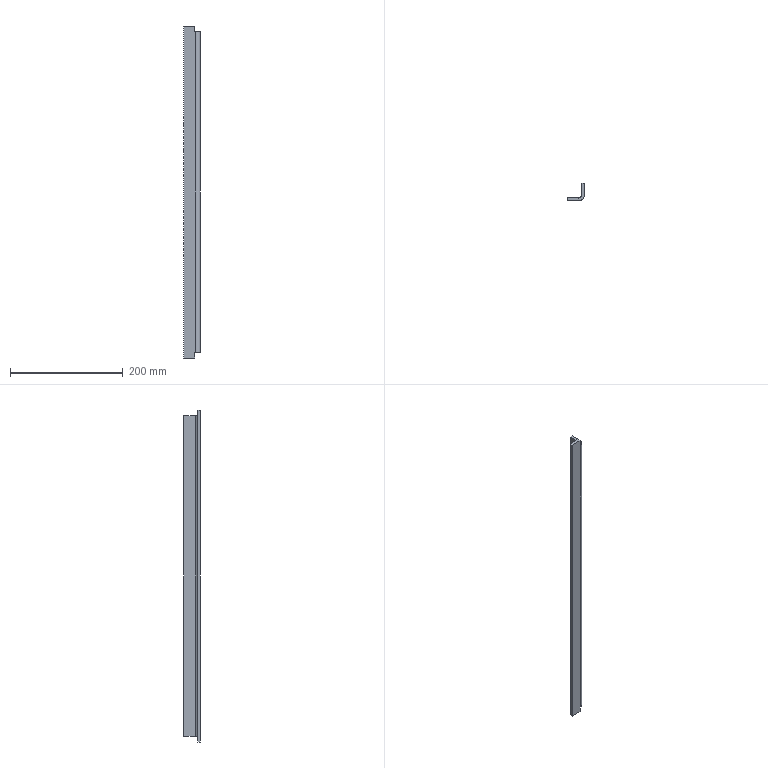Part | STEP file | PN_0019_bent angle steel | 1 solid | 14 faces | box 30 x 30 x 590 mm | volume 150799 mm3 | plane 12 | cylinder 2 | commonest cylinder face diameters 8 x1 18 x1
STEP:
#1=CARTESIAN_POINT('',(0.,0.,0.));
#2=DIRECTION('',(0.,0.,1.));
#3=DIRECTION('',(1.,0.,0.));
#4=AXIS2_PLACEMENT_3D('',#1,#2,#3);
#5=CARTESIAN_POINT('',(189.,-130.,10.));
#6=VERTEX_POINT('',#5);
#7=CARTESIAN_POINT('',(188.,-130.,10.));
#8=VERTEX_POINT('',#7);
#9=CARTESIAN_POINT('',(188.,-130.,10.));
#10=DIRECTION('',(-1.,0.,0.));
#11=VECTOR('',#10,1.);
#12=LINE('',#9,#11);
#13=CARTESIAN_POINT('',(198.,-130.,295.));
#14=DIRECTION('',(0.,-1.,0.));
#15=DIRECTION('',(0.,0.,-1.));
#16=AXIS2_PLACEMENT_3D('',#13,#14,#15);
#17=PLANE('',#16);
#18=CARTESIAN_POINT('',(285.,-10.));
#19=DIRECTION('',(0.,-1.));
#20=VECTOR('',#19,1.);
#21=LINE('',#18,#20);
#22=(GEOMETRIC_REPRESENTATION_CONTEXT(2)PARAMETRIC_REPRESENTATION_CONTEXT()REPRESENTATION_CONTEXT('',''));
#23=DEFINITIONAL_REPRESENTATION('',(#21),#22);
#24=PCURVE('',#17,#23);
#25=CARTESIAN_POINT('',(188.,-105.,10.));
#26=DIRECTION('',(0.,0.,1.));
#27=DIRECTION('',(0.,-1.,0.));
#28=AXIS2_PLACEMENT_3D('',#25,#26,#27);
#29=PLANE('',#28);
#30=CARTESIAN_POINT('',(25.,0.));
#31=DIRECTION('',(0.,-1.));
#32=VECTOR('',#31,1.);
#33=LINE('',#30,#32);
#34=(GEOMETRIC_REPRESENTATION_CONTEXT(2)PARAMETRIC_REPRESENTATION_CONTEXT()REPRESENTATION_CONTEXT('',''));
#35=DEFINITIONAL_REPRESENTATION('',(#33),#34);
#36=PCURVE('',#29,#35);
#37=SURFACE_CURVE('',#12,(#24,#36),.PCURVE_S1.);
#38=EDGE_CURVE('',#6,#8,#37,.T.);
#39=ORIENTED_EDGE('',*,*,#38,.T.);
#40=CARTESIAN_POINT('',(188.,-130.,0.));
#41=VERTEX_POINT('',#40);
#42=CARTESIAN_POINT('',(188.,-130.,295.));
#43=DIRECTION('',(0.,0.,1.));
#44=VECTOR('',#43,1.);
#45=LINE('',#42,#44);
#46=CARTESIAN_POINT('',(0.,-10.));
#47=DIRECTION('',(-1.,0.));
#48=VECTOR('',#47,1.);
#49=LINE('',#46,#48);
#50=(GEOMETRIC_REPRESENTATION_CONTEXT(2)PARAMETRIC_REPRESENTATION_CONTEXT()REPRESENTATION_CONTEXT('',''));
#51=DEFINITIONAL_REPRESENTATION('',(#49),#50);
#52=PCURVE('',#17,#51);
#53=CARTESIAN_POINT('',(188.,0.,0.));
#54=DIRECTION('',(-1.,0.,0.));
#55=DIRECTION('',(0.,0.,1.));
#56=AXIS2_PLACEMENT_3D('',#53,#54,#55);
#57=PLANE('',#56);
#58=CARTESIAN_POINT('',(295.,-130.));
#59=DIRECTION('',(1.,0.));
#60=VECTOR('',#59,1.);
#61=LINE('',#58,#60);
#62=(GEOMETRIC_REPRESENTATION_CONTEXT(2)PARAMETRIC_REPRESENTATION_CONTEXT()REPRESENTATION_CONTEXT('',''));
#63=DEFINITIONAL_REPRESENTATION('',(#61),#62);
#64=PCURVE('',#57,#63);
#65=SURFACE_CURVE('',#45,(#52,#64),.PCURVE_S1.);
#66=EDGE_CURVE('',#41,#8,#65,.T.);
#67=ORIENTED_EDGE('',*,*,#66,.F.);
#68=CARTESIAN_POINT('',(168.,-130.,0.));
#69=VERTEX_POINT('',#68);
#70=CARTESIAN_POINT('',(198.,-130.,0.));
#71=DIRECTION('',(1.,0.,0.));
#72=VECTOR('',#71,1.);
#73=LINE('',#70,#72);
#74=CARTESIAN_POINT('',(295.,0.));
#75=DIRECTION('',(0.,1.));
#76=VECTOR('',#75,1.);
#77=LINE('',#74,#76);
#78=(GEOMETRIC_REPRESENTATION_CONTEXT(2)PARAMETRIC_REPRESENTATION_CONTEXT()REPRESENTATION_CONTEXT('',''));
#79=DEFINITIONAL_REPRESENTATION('',(#77),#78);
#80=PCURVE('',#17,#79);
#81=CARTESIAN_POINT('',(189.,-126.,0.));
#82=DIRECTION('',(0.,0.,1.));
#83=DIRECTION('',(0.,-1.,0.));
#84=AXIS2_PLACEMENT_3D('',#81,#82,#83);
#85=PLANE('',#84);
#86=CARTESIAN_POINT('',(4.,9.));
#87=DIRECTION('',(0.,1.));
#88=VECTOR('',#87,1.);
#89=LINE('',#86,#88);
#90=(GEOMETRIC_REPRESENTATION_CONTEXT(2)PARAMETRIC_REPRESENTATION_CONTEXT()REPRESENTATION_CONTEXT('',''));
#91=DEFINITIONAL_REPRESENTATION('',(#89),#90);
#92=PCURVE('',#85,#91);
#93=SURFACE_CURVE('',#73,(#80,#92),.PCURVE_S1.);
#94=EDGE_CURVE('',#69,#41,#93,.T.);
#95=ORIENTED_EDGE('',*,*,#94,.F.);
#96=CARTESIAN_POINT('',(168.,-130.,590.));
#97=VERTEX_POINT('',#96);
#98=CARTESIAN_POINT('',(168.,-130.,295.));
#99=DIRECTION('',(0.,0.,-1.));
#100=VECTOR('',#99,1.);
#101=LINE('',#98,#100);
#102=CARTESIAN_POINT('',(0.,-30.));
#103=DIRECTION('',(1.,0.));
#104=VECTOR('',#103,1.);
#105=LINE('',#102,#104);
#106=(GEOMETRIC_REPRESENTATION_CONTEXT(2)PARAMETRIC_REPRESENTATION_CONTEXT()REPRESENTATION_CONTEXT('',''));
#107=DEFINITIONAL_REPRESENTATION('',(#105),#106);
#108=PCURVE('',#17,#107);
#109=CARTESIAN_POINT('',(168.,-135.,295.));
#110=DIRECTION('',(-1.,0.,0.));
#111=DIRECTION('',(0.,0.,1.));
#112=AXIS2_PLACEMENT_3D('',#109,#110,#111);
#113=PLANE('',#112);
#114=CARTESIAN_POINT('',(0.,5.));
#115=DIRECTION('',(-1.,0.));
#116=VECTOR('',#115,1.);
#117=LINE('',#114,#116);
#118=(GEOMETRIC_REPRESENTATION_CONTEXT(2)PARAMETRIC_REPRESENTATION_CONTEXT()REPRESENTATION_CONTEXT('',''));
#119=DEFINITIONAL_REPRESENTATION('',(#117),#118);
#120=PCURVE('',#113,#119);
#121=SURFACE_CURVE('',#101,(#108,#120),.PCURVE_S1.);
#122=EDGE_CURVE('',#97,#69,#121,.T.);
#123=ORIENTED_EDGE('',*,*,#122,.F.);
#124=CARTESIAN_POINT('',(188.,-130.,590.));
#125=VERTEX_POINT('',#124);
#126=CARTESIAN_POINT('',(198.,-130.,590.));
#127=DIRECTION('',(-1.,0.,0.));
#128=VECTOR('',#127,1.);
#129=LINE('',#126,#128);
#130=CARTESIAN_POINT('',(-295.,0.));
#131=DIRECTION('',(0.,-1.));
#132=VECTOR('',#131,1.);
#133=LINE('',#130,#132);
#134=(GEOMETRIC_REPRESENTATION_CONTEXT(2)PARAMETRIC_REPRESENTATION_CONTEXT()REPRESENTATION_CONTEXT('',''));
#135=DEFINITIONAL_REPRESENTATION('',(#133),#134);
#136=PCURVE('',#17,#135);
#137=CARTESIAN_POINT('',(189.,-126.,590.));
#138=DIRECTION('',(0.,0.,-1.));
#139=DIRECTION('',(0.,1.,0.));
#140=AXIS2_PLACEMENT_3D('',#137,#138,#139);
#141=PLANE('',#140);
#142=CARTESIAN_POINT('',(-4.,9.));
#143=DIRECTION('',(0.,-1.));
#144=VECTOR('',#143,1.);
#145=LINE('',#142,#144);
#146=(GEOMETRIC_REPRESENTATION_CONTEXT(2)PARAMETRIC_REPRESENTATION_CONTEXT()REPRESENTATION_CONTEXT('',''));
#147=DEFINITIONAL_REPRESENTATION('',(#145),#146);
#148=PCURVE('',#141,#147);
#149=SURFACE_CURVE('',#129,(#136,#148),.PCURVE_S1.);
#150=EDGE_CURVE('',#125,#97,#149,.T.);
#151=ORIENTED_EDGE('',*,*,#150,.F.);
#152=CARTESIAN_POINT('',(188.,-130.,580.));
#153=VERTEX_POINT('',#152);
#154=CARTESIAN_POINT('',(188.,-130.,295.));
#155=DIRECTION('',(0.,0.,1.));
#156=VECTOR('',#155,1.);
#157=LINE('',#154,#156);
#158=CARTESIAN_POINT('',(0.,-10.));
#159=DIRECTION('',(-1.,0.));
#160=VECTOR('',#159,1.);
#161=LINE('',#158,#160);
#162=(GEOMETRIC_REPRESENTATION_CONTEXT(2)PARAMETRIC_REPRESENTATION_CONTEXT()REPRESENTATION_CONTEXT('',''));
#163=DEFINITIONAL_REPRESENTATION('',(#161),#162);
#164=PCURVE('',#17,#163);
#165=CARTESIAN_POINT('',(188.,0.,590.));
#166=DIRECTION('',(-1.,0.,0.));
#167=DIRECTION('',(0.,0.,1.));
#168=AXIS2_PLACEMENT_3D('',#165,#166,#167);
#169=PLANE('',#168);
#170=CARTESIAN_POINT('',(-295.,-130.));
#171=DIRECTION('',(1.,0.));
#172=VECTOR('',#171,1.);
#173=LINE('',#170,#172);
#174=(GEOMETRIC_REPRESENTATION_CONTEXT(2)PARAMETRIC_REPRESENTATION_CONTEXT()REPRESENTATION_CONTEXT('',''));
#175=DEFINITIONAL_REPRESENTATION('',(#173),#174);
#176=PCURVE('',#169,#175);
#177=SURFACE_CURVE('',#157,(#164,#176),.PCURVE_S1.);
#178=EDGE_CURVE('',#153,#125,#177,.T.);
#179=ORIENTED_EDGE('',*,*,#178,.F.);
#180=CARTESIAN_POINT('',(189.,-130.,580.));
#181=VERTEX_POINT('',#180);
#182=CARTESIAN_POINT('',(188.,-130.,580.));
#183=DIRECTION('',(1.,0.,0.));
#184=VECTOR('',#183,1.);
#185=LINE('',#182,#184);
#186=CARTESIAN_POINT('',(-285.,-10.));
#187=DIRECTION('',(0.,1.));
#188=VECTOR('',#187,1.);
#189=LINE('',#186,#188);
#190=(GEOMETRIC_REPRESENTATION_CONTEXT(2)PARAMETRIC_REPRESENTATION_CONTEXT()REPRESENTATION_CONTEXT('',''));
#191=DEFINITIONAL_REPRESENTATION('',(#189),#190);
#192=PCURVE('',#17,#191);
#193=CARTESIAN_POINT('',(188.,-105.,580.));
#194=DIRECTION('',(0.,0.,-1.));
#195=DIRECTION('',(0.,1.,0.));
#196=AXIS2_PLACEMENT_3D('',#193,#194,#195);
#197=PLANE('',#196);
#198=CARTESIAN_POINT('',(-25.,0.));
#199=DIRECTION('',(0.,1.));
#200=VECTOR('',#199,1.);
#201=LINE('',#198,#200);
#202=(GEOMETRIC_REPRESENTATION_CONTEXT(2)PARAMETRIC_REPRESENTATION_CONTEXT()REPRESENTATION_CONTEXT('',''));
#203=DEFINITIONAL_REPRESENTATION('',(#201),#202);
#204=PCURVE('',#197,#203);
#205=SURFACE_CURVE('',#185,(#192,#204),.PCURVE_S1.);
#206=EDGE_CURVE('',#153,#181,#205,.T.);
#207=ORIENTED_EDGE('',*,*,#206,.T.);
#208=CARTESIAN_POINT('',(189.,-130.,295.));
#209=DIRECTION('',(0.,0.,1.));
#210=VECTOR('',#209,1.);
#211=LINE('',#208,#210);
#212=CARTESIAN_POINT('',(0.,-9.));
#213=DIRECTION('',(-1.,0.));
#214=VECTOR('',#213,1.);
#215=LINE('',#212,#214);
#216=(GEOMETRIC_REPRESENTATION_CONTEXT(2)PARAMETRIC_REPRESENTATION_CONTEXT()REPRESENTATION_CONTEXT('',''));
#217=DEFINITIONAL_REPRESENTATION('',(#215),#216);
#218=PCURVE('',#17,#217);
#219=CARTESIAN_POINT('',(189.,-126.,295.));
#220=DIRECTION('',(0.,0.,-1.));
#221=DIRECTION('',(0.,1.,0.));
#222=AXIS2_PLACEMENT_3D('',#219,#220,#221);
#223=CYLINDRICAL_SURFACE('',#222,4.);
#224=CARTESIAN_POINT('',(3.142,0.));
#225=DIRECTION('',(0.,-1.));
#226=VECTOR('',#225,1.);
#227=LINE('',#224,#226);
#228=(GEOMETRIC_REPRESENTATION_CONTEXT(2)PARAMETRIC_REPRESENTATION_CONTEXT()REPRESENTATION_CONTEXT('',''));
#229=DEFINITIONAL_REPRESENTATION('',(#227),#228);
#230=PCURVE('',#223,#229);
#231=SURFACE_CURVE('',#211,(#218,#230),.PCURVE_S1.);
#232=EDGE_CURVE('',#6,#181,#231,.T.);
#233=ORIENTED_EDGE('',*,*,#232,.F.);
#234=EDGE_LOOP('',(#39,#67,#95,#123,#151,#179,#207,#233));
#235=FACE_BOUND('',#234,.T.);
#236=ADVANCED_FACE('',(#235),#17,.F.);
#237=CARTESIAN_POINT('',(193.,-126.,10.));
#238=VERTEX_POINT('',#237);
#239=CARTESIAN_POINT('',(193.,-126.,580.));
#240=VERTEX_POINT('',#239);
#241=CARTESIAN_POINT('',(193.,-126.,295.));
#242=DIRECTION('',(0.,0.,1.));
#243=VECTOR('',#242,1.);
#244=LINE('',#241,#243);
#245=CARTESIAN_POINT('',(1.571,0.));
#246=DIRECTION('',(0.,-1.));
#247=VECTOR('',#246,1.);
#248=LINE('',#245,#247);
#249=(GEOMETRIC_REPRESENTATION_CONTEXT(2)PARAMETRIC_REPRESENTATION_CONTEXT()REPRESENTATION_CONTEXT('',''));
#250=DEFINITIONAL_REPRESENTATION('',(#248),#249);
#251=PCURVE('',#223,#250);
#252=CARTESIAN_POINT('',(193.,-105.,295.));
#253=DIRECTION('',(1.,0.,0.));
#254=DIRECTION('',(0.,0.,-1.));
#255=AXIS2_PLACEMENT_3D('',#252,#253,#254);
#256=PLANE('',#255);
#257=CARTESIAN_POINT('',(0.,-21.));
#258=DIRECTION('',(-1.,0.));
#259=VECTOR('',#258,1.);
#260=LINE('',#257,#259);
#261=(GEOMETRIC_REPRESENTATION_CONTEXT(2)PARAMETRIC_REPRESENTATION_CONTEXT()REPRESENTATION_CONTEXT('',''));
#262=DEFINITIONAL_REPRESENTATION('',(#260),#261);
#263=PCURVE('',#256,#262);
#264=SURFACE_CURVE('',#244,(#251,#263),.PCURVE_S1.);
#265=EDGE_CURVE('',#238,#240,#264,.T.);
#266=ORIENTED_EDGE('',*,*,#265,.T.);
#267=CARTESIAN_POINT('',(189.,-126.,580.));
#268=DIRECTION('',(0.,0.,-1.));
#269=DIRECTION('',(0.,1.,0.));
#270=AXIS2_PLACEMENT_3D('',#267,#268,#269);
#271=CIRCLE('',#270,4.);
#272=CARTESIAN_POINT('',(0.,-285.));
#273=DIRECTION('',(1.,0.));
#274=VECTOR('',#273,1.);
#275=LINE('',#272,#274);
#276=(GEOMETRIC_REPRESENTATION_CONTEXT(2)PARAMETRIC_REPRESENTATION_CONTEXT()REPRESENTATION_CONTEXT('',''));
#277=DEFINITIONAL_REPRESENTATION('',(#275),#276);
#278=PCURVE('',#223,#277);
#279=CARTESIAN_POINT('',(-21.,1.));
#280=DIRECTION('',(1.,0.));
#281=AXIS2_PLACEMENT_2D('',#279,#280);
#282=CIRCLE('',#281,4.);
#283=(GEOMETRIC_REPRESENTATION_CONTEXT(2)PARAMETRIC_REPRESENTATION_CONTEXT()REPRESENTATION_CONTEXT('',''));
#284=DEFINITIONAL_REPRESENTATION('',(#282),#283);
#285=PCURVE('',#197,#284);
#286=SURFACE_CURVE('',#271,(#278,#285),.PCURVE_S1.);
#287=EDGE_CURVE('',#240,#181,#286,.T.);
#288=ORIENTED_EDGE('',*,*,#287,.T.);
#289=ORIENTED_EDGE('',*,*,#232,.F.);
#290=CARTESIAN_POINT('',(189.,-126.,10.));
#291=DIRECTION('',(0.,0.,1.));
#292=DIRECTION('',(0.,1.,0.));
#293=AXIS2_PLACEMENT_3D('',#290,#291,#292);
#294=CIRCLE('',#293,4.);
#295=CARTESIAN_POINT('',(6.283,285.));
#296=DIRECTION('',(-1.,0.));
#297=VECTOR('',#296,1.);
#298=LINE('',#295,#297);
#299=(GEOMETRIC_REPRESENTATION_CONTEXT(2)PARAMETRIC_REPRESENTATION_CONTEXT()REPRESENTATION_CONTEXT('',''));
#300=DEFINITIONAL_REPRESENTATION('',(#298),#299);
#301=PCURVE('',#223,#300);
#302=CARTESIAN_POINT('',(21.,1.));
#303=DIRECTION('',(-1.,0.));
#304=AXIS2_PLACEMENT_2D('',#302,#303);
#305=CIRCLE('',#304,4.);
#306=(GEOMETRIC_REPRESENTATION_CONTEXT(2)PARAMETRIC_REPRESENTATION_CONTEXT()REPRESENTATION_CONTEXT('',''));
#307=DEFINITIONAL_REPRESENTATION('',(#305),#306);
#308=PCURVE('',#29,#307);
#309=SURFACE_CURVE('',#294,(#301,#308),.PCURVE_S1.);
#310=EDGE_CURVE('',#6,#238,#309,.T.);
#311=ORIENTED_EDGE('',*,*,#310,.T.);
#312=EDGE_LOOP('',(#266,#288,#289,#311));
#313=FACE_BOUND('',#312,.F.);
#314=ADVANCED_FACE('',(#313),#223,.F.);
#315=CARTESIAN_POINT('',(188.,-135.,0.));
#316=VERTEX_POINT('',#315);
#317=CARTESIAN_POINT('',(188.,-135.,10.));
#318=VERTEX_POINT('',#317);
#319=CARTESIAN_POINT('',(188.,-135.,0.));
#320=DIRECTION('',(0.,0.,1.));
#321=VECTOR('',#320,1.);
#322=LINE('',#319,#321);
#323=CARTESIAN_POINT('',(0.,-135.));
#324=DIRECTION('',(1.,0.));
#325=VECTOR('',#324,1.);
#326=LINE('',#323,#325);
#327=(GEOMETRIC_REPRESENTATION_CONTEXT(2)PARAMETRIC_REPRESENTATION_CONTEXT()REPRESENTATION_CONTEXT('',''));
#328=DEFINITIONAL_REPRESENTATION('',(#326),#327);
#329=PCURVE('',#57,#328);
#330=CARTESIAN_POINT('',(198.,-135.,295.));
#331=DIRECTION('',(0.,-1.,0.));
#332=DIRECTION('',(0.,0.,-1.));
#333=AXIS2_PLACEMENT_3D('',#330,#331,#332);
#334=PLANE('',#333);
#335=CARTESIAN_POINT('',(295.,-10.));
#336=DIRECTION('',(-1.,0.));
#337=VECTOR('',#336,1.);
#338=LINE('',#335,#337);
#339=(GEOMETRIC_REPRESENTATION_CONTEXT(2)PARAMETRIC_REPRESENTATION_CONTEXT()REPRESENTATION_CONTEXT('',''));
#340=DEFINITIONAL_REPRESENTATION('',(#338),#339);
#341=PCURVE('',#334,#340);
#342=SURFACE_CURVE('',#322,(#329,#341),.PCURVE_S1.);
#343=EDGE_CURVE('',#316,#318,#342,.T.);
#344=ORIENTED_EDGE('',*,*,#343,.F.);
#345=CARTESIAN_POINT('',(188.,0.,0.));
#346=DIRECTION('',(0.,-1.,0.));
#347=VECTOR('',#346,1.);
#348=LINE('',#345,#347);
#349=CARTESIAN_POINT('',(0.,0.));
#350=DIRECTION('',(0.,-1.));
#351=VECTOR('',#350,1.);
#352=LINE('',#349,#351);
#353=(GEOMETRIC_REPRESENTATION_CONTEXT(2)PARAMETRIC_REPRESENTATION_CONTEXT()REPRESENTATION_CONTEXT('',''));
#354=DEFINITIONAL_REPRESENTATION('',(#352),#353);
#355=PCURVE('',#57,#354);
#356=CARTESIAN_POINT('',(-126.,-1.));
#357=DIRECTION('',(1.,0.));
#358=VECTOR('',#357,1.);
#359=LINE('',#356,#358);
#360=(GEOMETRIC_REPRESENTATION_CONTEXT(2)PARAMETRIC_REPRESENTATION_CONTEXT()REPRESENTATION_CONTEXT('',''));
#361=DEFINITIONAL_REPRESENTATION('',(#359),#360);
#362=PCURVE('',#85,#361);
#363=SURFACE_CURVE('',#348,(#355,#362),.PCURVE_S1.);
#364=EDGE_CURVE('',#41,#316,#363,.T.);
#365=ORIENTED_EDGE('',*,*,#364,.F.);
#366=ORIENTED_EDGE('',*,*,#66,.T.);
#367=CARTESIAN_POINT('',(188.,0.,10.));
#368=DIRECTION('',(0.,1.,0.));
#369=VECTOR('',#368,1.);
#370=LINE('',#367,#369);
#371=CARTESIAN_POINT('',(10.,0.));
#372=DIRECTION('',(0.,1.));
#373=VECTOR('',#372,1.);
#374=LINE('',#371,#373);
#375=(GEOMETRIC_REPRESENTATION_CONTEXT(2)PARAMETRIC_REPRESENTATION_CONTEXT()REPRESENTATION_CONTEXT('',''));
#376=DEFINITIONAL_REPRESENTATION('',(#374),#375);
#377=PCURVE('',#57,#376);
#378=CARTESIAN_POINT('',(-105.,0.));
#379=DIRECTION('',(-1.,0.));
#380=VECTOR('',#379,1.);
#381=LINE('',#378,#380);
#382=(GEOMETRIC_REPRESENTATION_CONTEXT(2)PARAMETRIC_REPRESENTATION_CONTEXT()REPRESENTATION_CONTEXT('',''));
#383=DEFINITIONAL_REPRESENTATION('',(#381),#382);
#384=PCURVE('',#29,#383);
#385=SURFACE_CURVE('',#370,(#377,#384),.PCURVE_S1.);
#386=EDGE_CURVE('',#318,#8,#385,.T.);
#387=ORIENTED_EDGE('',*,*,#386,.F.);
#388=EDGE_LOOP('',(#344,#365,#366,#387));
#389=FACE_BOUND('',#388,.T.);
#390=ADVANCED_FACE('',(#389),#57,.F.);
#391=ORIENTED_EDGE('',*,*,#364,.T.);
#392=CARTESIAN_POINT('',(168.,-135.,0.));
#393=VERTEX_POINT('',#392);
#394=CARTESIAN_POINT('',(189.,-135.,0.));
#395=DIRECTION('',(1.,0.,0.));
#396=VECTOR('',#395,1.);
#397=LINE('',#394,#396);
#398=CARTESIAN_POINT('',(9.,0.));
#399=DIRECTION('',(0.,1.));
#400=VECTOR('',#399,1.);
#401=LINE('',#398,#400);
#402=(GEOMETRIC_REPRESENTATION_CONTEXT(2)PARAMETRIC_REPRESENTATION_CONTEXT()REPRESENTATION_CONTEXT('',''));
#403=DEFINITIONAL_REPRESENTATION('',(#401),#402);
#404=PCURVE('',#85,#403);
#405=CARTESIAN_POINT('',(295.,-9.));
#406=DIRECTION('',(0.,1.));
#407=VECTOR('',#406,1.);
#408=LINE('',#405,#407);
#409=(GEOMETRIC_REPRESENTATION_CONTEXT(2)PARAMETRIC_REPRESENTATION_CONTEXT()REPRESENTATION_CONTEXT('',''));
#410=DEFINITIONAL_REPRESENTATION('',(#408),#409);
#411=PCURVE('',#334,#410);
#412=SURFACE_CURVE('',#397,(#404,#411),.PCURVE_S1.);
#413=EDGE_CURVE('',#393,#316,#412,.T.);
#414=ORIENTED_EDGE('',*,*,#413,.F.);
#415=CARTESIAN_POINT('',(168.,-126.,0.));
#416=DIRECTION('',(0.,-1.,0.));
#417=VECTOR('',#416,1.);
#418=LINE('',#415,#417);
#419=CARTESIAN_POINT('',(0.,-21.));
#420=DIRECTION('',(1.,0.));
#421=VECTOR('',#420,1.);
#422=LINE('',#419,#421);
#423=(GEOMETRIC_REPRESENTATION_CONTEXT(2)PARAMETRIC_REPRESENTATION_CONTEXT()REPRESENTATION_CONTEXT('',''));
#424=DEFINITIONAL_REPRESENTATION('',(#422),#423);
#425=PCURVE('',#85,#424);
#426=CARTESIAN_POINT('',(-295.,9.));
#427=DIRECTION('',(0.,-1.));
#428=VECTOR('',#427,1.);
#429=LINE('',#426,#428);
#430=(GEOMETRIC_REPRESENTATION_CONTEXT(2)PARAMETRIC_REPRESENTATION_CONTEXT()REPRESENTATION_CONTEXT('',''));
#431=DEFINITIONAL_REPRESENTATION('',(#429),#430);
#432=PCURVE('',#113,#431);
#433=SURFACE_CURVE('',#418,(#425,#432),.PCURVE_S1.);
#434=EDGE_CURVE('',#69,#393,#433,.T.);
#435=ORIENTED_EDGE('',*,*,#434,.F.);
#436=ORIENTED_EDGE('',*,*,#94,.T.);
#437=EDGE_LOOP('',(#391,#414,#435,#436));
#438=FACE_BOUND('',#437,.T.);
#439=ADVANCED_FACE('',(#438),#85,.F.);
#440=CARTESIAN_POINT('',(168.,-135.,590.));
#441=VERTEX_POINT('',#440);
#442=CARTESIAN_POINT('',(168.,-135.,590.));
#443=DIRECTION('',(0.,1.,0.));
#444=VECTOR('',#443,1.);
#445=LINE('',#442,#444);
#446=CARTESIAN_POINT('',(295.,0.));
#447=DIRECTION('',(0.,1.));
#448=VECTOR('',#447,1.);
#449=LINE('',#446,#448);
#450=(GEOMETRIC_REPRESENTATION_CONTEXT(2)PARAMETRIC_REPRESENTATION_CONTEXT()REPRESENTATION_CONTEXT('',''));
#451=DEFINITIONAL_REPRESENTATION('',(#449),#450);
#452=PCURVE('',#113,#451);
#453=CARTESIAN_POINT('',(-9.,-21.));
#454=DIRECTION('',(1.,0.));
#455=VECTOR('',#454,1.);
#456=LINE('',#453,#455);
#457=(GEOMETRIC_REPRESENTATION_CONTEXT(2)PARAMETRIC_REPRESENTATION_CONTEXT()REPRESENTATION_CONTEXT('',''));
#458=DEFINITIONAL_REPRESENTATION('',(#456),#457);
#459=PCURVE('',#141,#458);
#460=SURFACE_CURVE('',#445,(#452,#459),.PCURVE_S1.);
#461=EDGE_CURVE('',#441,#97,#460,.T.);
#462=ORIENTED_EDGE('',*,*,#461,.T.);
#463=ORIENTED_EDGE('',*,*,#122,.T.);
#464=ORIENTED_EDGE('',*,*,#434,.T.);
#465=CARTESIAN_POINT('',(168.,-135.,295.));
#466=DIRECTION('',(0.,0.,1.));
#467=VECTOR('',#466,1.);
#468=LINE('',#465,#467);
#469=CARTESIAN_POINT('',(0.,0.));
#470=DIRECTION('',(1.,0.));
#471=VECTOR('',#470,1.);
#472=LINE('',#469,#471);
#473=(GEOMETRIC_REPRESENTATION_CONTEXT(2)PARAMETRIC_REPRESENTATION_CONTEXT()REPRESENTATION_CONTEXT('',''));
#474=DEFINITIONAL_REPRESENTATION('',(#472),#473);
#475=PCURVE('',#113,#474);
#476=CARTESIAN_POINT('',(0.,-30.));
#477=DIRECTION('',(-1.,0.));
#478=VECTOR('',#477,1.);
#479=LINE('',#476,#478);
#480=(GEOMETRIC_REPRESENTATION_CONTEXT(2)PARAMETRIC_REPRESENTATION_CONTEXT()REPRESENTATION_CONTEXT('',''));
#481=DEFINITIONAL_REPRESENTATION('',(#479),#480);
#482=PCURVE('',#334,#481);
#483=SURFACE_CURVE('',#468,(#475,#482),.PCURVE_S1.);
#484=EDGE_CURVE('',#393,#441,#483,.T.);
#485=ORIENTED_EDGE('',*,*,#484,.T.);
#486=EDGE_LOOP('',(#462,#463,#464,#485));
#487=FACE_BOUND('',#486,.T.);
#488=ADVANCED_FACE('',(#487),#113,.T.);
#489=ORIENTED_EDGE('',*,*,#461,.F.);
#490=CARTESIAN_POINT('',(188.,-135.,590.));
#491=VERTEX_POINT('',#490);
#492=CARTESIAN_POINT('',(189.,-135.,590.));
#493=DIRECTION('',(-1.,0.,0.));
#494=VECTOR('',#493,1.);
#495=LINE('',#492,#494);
#496=CARTESIAN_POINT('',(-9.,0.));
#497=DIRECTION('',(0.,-1.));
#498=VECTOR('',#497,1.);
#499=LINE('',#496,#498);
#500=(GEOMETRIC_REPRESENTATION_CONTEXT(2)PARAMETRIC_REPRESENTATION_CONTEXT()REPRESENTATION_CONTEXT('',''));
#501=DEFINITIONAL_REPRESENTATION('',(#499),#500);
#502=PCURVE('',#141,#501);
#503=CARTESIAN_POINT('',(-295.,-9.));
#504=DIRECTION('',(0.,-1.));
#505=VECTOR('',#504,1.);
#506=LINE('',#503,#505);
#507=(GEOMETRIC_REPRESENTATION_CONTEXT(2)PARAMETRIC_REPRESENTATION_CONTEXT()REPRESENTATION_CONTEXT('',''));
#508=DEFINITIONAL_REPRESENTATION('',(#506),#507);
#509=PCURVE('',#334,#508);
#510=SURFACE_CURVE('',#495,(#502,#509),.PCURVE_S1.);
#511=EDGE_CURVE('',#491,#441,#510,.T.);
#512=ORIENTED_EDGE('',*,*,#511,.F.);
#513=CARTESIAN_POINT('',(188.,-126.,590.));
#514=DIRECTION('',(0.,-1.,0.));
#515=VECTOR('',#514,1.);
#516=LINE('',#513,#515);
#517=CARTESIAN_POINT('',(0.,-1.));
#518=DIRECTION('',(-1.,0.));
#519=VECTOR('',#518,1.);
#520=LINE('',#517,#519);
#521=(GEOMETRIC_REPRESENTATION_CONTEXT(2)PARAMETRIC_REPRESENTATION_CONTEXT()REPRESENTATION_CONTEXT('',''));
#522=DEFINITIONAL_REPRESENTATION('',(#520),#521);
#523=PCURVE('',#141,#522);
#524=CARTESIAN_POINT('',(0.,-126.));
#525=DIRECTION('',(0.,-1.));
#526=VECTOR('',#525,1.);
#527=LINE('',#524,#526);
#528=(GEOMETRIC_REPRESENTATION_CONTEXT(2)PARAMETRIC_REPRESENTATION_CONTEXT()REPRESENTATION_CONTEXT('',''));
#529=DEFINITIONAL_REPRESENTATION('',(#527),#528);
#530=PCURVE('',#169,#529);
#531=SURFACE_CURVE('',#516,(#523,#530),.PCURVE_S1.);
#532=EDGE_CURVE('',#125,#491,#531,.T.);
#533=ORIENTED_EDGE('',*,*,#532,.F.);
#534=ORIENTED_EDGE('',*,*,#150,.T.);
#535=EDGE_LOOP('',(#489,#512,#533,#534));
#536=FACE_BOUND('',#535,.T.);
#537=ADVANCED_FACE('',(#536),#141,.F.);
#538=ORIENTED_EDGE('',*,*,#178,.T.);
#539=ORIENTED_EDGE('',*,*,#532,.T.);
#540=CARTESIAN_POINT('',(188.,-135.,580.));
#541=VERTEX_POINT('',#540);
#542=CARTESIAN_POINT('',(188.,-135.,590.));
#543=DIRECTION('',(0.,0.,1.));
#544=VECTOR('',#543,1.);
#545=LINE('',#542,#544);
#546=CARTESIAN_POINT('',(0.,-135.));
#547=DIRECTION('',(1.,0.));
#548=VECTOR('',#547,1.);
#549=LINE('',#546,#548);
#550=(GEOMETRIC_REPRESENTATION_CONTEXT(2)PARAMETRIC_REPRESENTATION_CONTEXT()REPRESENTATION_CONTEXT('',''));
#551=DEFINITIONAL_REPRESENTATION('',(#549),#550);
#552=PCURVE('',#169,#551);
#553=CARTESIAN_POINT('',(-295.,-10.));
#554=DIRECTION('',(-1.,0.));
#555=VECTOR('',#554,1.);
#556=LINE('',#553,#555);
#557=(GEOMETRIC_REPRESENTATION_CONTEXT(2)PARAMETRIC_REPRESENTATION_CONTEXT()REPRESENTATION_CONTEXT('',''));
#558=DEFINITIONAL_REPRESENTATION('',(#556),#557);
#559=PCURVE('',#334,#558);
#560=SURFACE_CURVE('',#545,(#552,#559),.PCURVE_S1.);
#561=EDGE_CURVE('',#541,#491,#560,.T.);
#562=ORIENTED_EDGE('',*,*,#561,.F.);
#563=CARTESIAN_POINT('',(188.,0.,580.));
#564=DIRECTION('',(0.,-1.,0.));
#565=VECTOR('',#564,1.);
#566=LINE('',#563,#565);
#567=CARTESIAN_POINT('',(-10.,0.));
#568=DIRECTION('',(0.,-1.));
#569=VECTOR('',#568,1.);
#570=LINE('',#567,#569);
#571=(GEOMETRIC_REPRESENTATION_CONTEXT(2)PARAMETRIC_REPRESENTATION_CONTEXT()REPRESENTATION_CONTEXT('',''));
#572=DEFINITIONAL_REPRESENTATION('',(#570),#571);
#573=PCURVE('',#169,#572);
#574=CARTESIAN_POINT('',(105.,0.));
#575=DIRECTION('',(-1.,0.));
#576=VECTOR('',#575,1.);
#577=LINE('',#574,#576);
#578=(GEOMETRIC_REPRESENTATION_CONTEXT(2)PARAMETRIC_REPRESENTATION_CONTEXT()REPRESENTATION_CONTEXT('',''));
#579=DEFINITIONAL_REPRESENTATION('',(#577),#578);
#580=PCURVE('',#197,#579);
#581=SURFACE_CURVE('',#566,(#573,#580),.PCURVE_S1.);
#582=EDGE_CURVE('',#153,#541,#581,.T.);
#583=ORIENTED_EDGE('',*,*,#582,.F.);
#584=EDGE_LOOP('',(#538,#539,#562,#583));
#585=FACE_BOUND('',#584,.T.);
#586=ADVANCED_FACE('',(#585),#169,.F.);
#587=CARTESIAN_POINT('',(193.,-105.,10.));
#588=VERTEX_POINT('',#587);
#589=CARTESIAN_POINT('',(193.,-105.,10.));
#590=DIRECTION('',(0.,1.,0.));
#591=VECTOR('',#590,1.);
#592=LINE('',#589,#591);
#593=CARTESIAN_POINT('',(285.,0.));
#594=DIRECTION('',(0.,1.));
#595=VECTOR('',#594,1.);
#596=LINE('',#593,#595);
#597=(GEOMETRIC_REPRESENTATION_CONTEXT(2)PARAMETRIC_REPRESENTATION_CONTEXT()REPRESENTATION_CONTEXT('',''));
#598=DEFINITIONAL_REPRESENTATION('',(#596),#597);
#599=PCURVE('',#256,#598);
#600=CARTESIAN_POINT('',(0.,5.));
#601=DIRECTION('',(-1.,0.));
#602=VECTOR('',#601,1.);
#603=LINE('',#600,#602);
#604=(GEOMETRIC_REPRESENTATION_CONTEXT(2)PARAMETRIC_REPRESENTATION_CONTEXT()REPRESENTATION_CONTEXT('',''));
#605=DEFINITIONAL_REPRESENTATION('',(#603),#604);
#606=PCURVE('',#29,#605);
#607=SURFACE_CURVE('',#592,(#599,#606),.PCURVE_S1.);
#608=EDGE_CURVE('',#238,#588,#607,.T.);
#609=ORIENTED_EDGE('',*,*,#608,.F.);
#610=ORIENTED_EDGE('',*,*,#265,.T.);
#611=CARTESIAN_POINT('',(193.,-105.,580.));
#612=VERTEX_POINT('',#611);
#613=CARTESIAN_POINT('',(193.,-105.,580.));
#614=DIRECTION('',(0.,-1.,0.));
#615=VECTOR('',#614,1.);
#616=LINE('',#613,#615);
#617=CARTESIAN_POINT('',(-285.,0.));
#618=DIRECTION('',(0.,-1.));
#619=VECTOR('',#618,1.);
#620=LINE('',#617,#619);
#621=(GEOMETRIC_REPRESENTATION_CONTEXT(2)PARAMETRIC_REPRESENTATION_CONTEXT()REPRESENTATION_CONTEXT('',''));
#622=DEFINITIONAL_REPRESENTATION('',(#620),#621);
#623=PCURVE('',#256,#622);
#624=CARTESIAN_POINT('',(0.,5.));
#625=DIRECTION('',(-1.,0.));
#626=VECTOR('',#625,1.);
#627=LINE('',#624,#626);
#628=(GEOMETRIC_REPRESENTATION_CONTEXT(2)PARAMETRIC_REPRESENTATION_CONTEXT()REPRESENTATION_CONTEXT('',''));
#629=DEFINITIONAL_REPRESENTATION('',(#627),#628);
#630=PCURVE('',#197,#629);
#631=SURFACE_CURVE('',#616,(#623,#630),.PCURVE_S1.);
#632=EDGE_CURVE('',#612,#240,#631,.T.);
#633=ORIENTED_EDGE('',*,*,#632,.F.);
#634=CARTESIAN_POINT('',(193.,-105.,295.));
#635=DIRECTION('',(0.,0.,1.));
#636=VECTOR('',#635,1.);
#637=LINE('',#634,#636);
#638=CARTESIAN_POINT('',(0.,0.));
#639=DIRECTION('',(-1.,0.));
#640=VECTOR('',#639,1.);
#641=LINE('',#638,#640);
#642=(GEOMETRIC_REPRESENTATION_CONTEXT(2)PARAMETRIC_REPRESENTATION_CONTEXT()REPRESENTATION_CONTEXT('',''));
#643=DEFINITIONAL_REPRESENTATION('',(#641),#642);
#644=PCURVE('',#256,#643);
#645=CARTESIAN_POINT('',(193.,-105.,295.));
#646=DIRECTION('',(0.,1.,0.));
#647=DIRECTION('',(0.,0.,1.));
#648=AXIS2_PLACEMENT_3D('',#645,#646,#647);
#649=PLANE('',#648);
#650=CARTESIAN_POINT('',(0.,0.));
#651=DIRECTION('',(1.,0.));
#652=VECTOR('',#651,1.);
#653=LINE('',#650,#652);
#654=(GEOMETRIC_REPRESENTATION_CONTEXT(2)PARAMETRIC_REPRESENTATION_CONTEXT()REPRESENTATION_CONTEXT('',''));
#655=DEFINITIONAL_REPRESENTATION('',(#653),#654);
#656=PCURVE('',#649,#655);
#657=SURFACE_CURVE('',#637,(#644,#656),.PCURVE_S1.);
#658=EDGE_CURVE('',#588,#612,#657,.T.);
#659=ORIENTED_EDGE('',*,*,#658,.F.);
#660=EDGE_LOOP('',(#609,#610,#633,#659));
#661=FACE_BOUND('',#660,.T.);
#662=ADVANCED_FACE('',(#661),#256,.F.);
#663=CARTESIAN_POINT('',(189.,-135.,10.));
#664=VERTEX_POINT('',#663);
#665=CARTESIAN_POINT('',(198.,-126.,10.));
#666=VERTEX_POINT('',#665);
#667=CARTESIAN_POINT('',(189.,-126.,10.));
#668=DIRECTION('',(0.,0.,1.));
#669=DIRECTION('',(0.,1.,0.));
#670=AXIS2_PLACEMENT_3D('',#667,#668,#669);
#671=CIRCLE('',#670,9.);
#672=CARTESIAN_POINT('',(21.,1.));
#673=DIRECTION('',(-1.,0.));
#674=AXIS2_PLACEMENT_2D('',#672,#673);
#675=CIRCLE('',#674,9.);
#676=(GEOMETRIC_REPRESENTATION_CONTEXT(2)PARAMETRIC_REPRESENTATION_CONTEXT()REPRESENTATION_CONTEXT('',''));
#677=DEFINITIONAL_REPRESENTATION('',(#675),#676);
#678=PCURVE('',#29,#677);
#679=CARTESIAN_POINT('',(189.,-126.,295.));
#680=DIRECTION('',(0.,0.,-1.));
#681=DIRECTION('',(0.,1.,0.));
#682=AXIS2_PLACEMENT_3D('',#679,#680,#681);
#683=CYLINDRICAL_SURFACE('',#682,9.);
#684=CARTESIAN_POINT('',(6.283,285.));
#685=DIRECTION('',(-1.,0.));
#686=VECTOR('',#685,1.);
#687=LINE('',#684,#686);
#688=(GEOMETRIC_REPRESENTATION_CONTEXT(2)PARAMETRIC_REPRESENTATION_CONTEXT()REPRESENTATION_CONTEXT('',''));
#689=DEFINITIONAL_REPRESENTATION('',(#687),#688);
#690=PCURVE('',#683,#689);
#691=SURFACE_CURVE('',#671,(#678,#690),.PCURVE_S1.);
#692=EDGE_CURVE('',#664,#666,#691,.T.);
#693=ORIENTED_EDGE('',*,*,#692,.F.);
#694=CARTESIAN_POINT('',(188.,-135.,10.));
#695=DIRECTION('',(1.,0.,0.));
#696=VECTOR('',#695,1.);
#697=LINE('',#694,#696);
#698=CARTESIAN_POINT('',(30.,0.));
#699=DIRECTION('',(0.,1.));
#700=VECTOR('',#699,1.);
#701=LINE('',#698,#700);
#702=(GEOMETRIC_REPRESENTATION_CONTEXT(2)PARAMETRIC_REPRESENTATION_CONTEXT()REPRESENTATION_CONTEXT('',''));
#703=DEFINITIONAL_REPRESENTATION('',(#701),#702);
#704=PCURVE('',#29,#703);
#705=CARTESIAN_POINT('',(285.,-10.));
#706=DIRECTION('',(0.,1.));
#707=VECTOR('',#706,1.);
#708=LINE('',#705,#707);
#709=(GEOMETRIC_REPRESENTATION_CONTEXT(2)PARAMETRIC_REPRESENTATION_CONTEXT()REPRESENTATION_CONTEXT('',''));
#710=DEFINITIONAL_REPRESENTATION('',(#708),#709);
#711=PCURVE('',#334,#710);
#712=SURFACE_CURVE('',#697,(#704,#711),.PCURVE_S1.);
#713=EDGE_CURVE('',#318,#664,#712,.T.);
#714=ORIENTED_EDGE('',*,*,#713,.F.);
#715=ORIENTED_EDGE('',*,*,#386,.T.);
#716=ORIENTED_EDGE('',*,*,#38,.F.);
#717=ORIENTED_EDGE('',*,*,#310,.T.);
#718=ORIENTED_EDGE('',*,*,#608,.T.);
#719=CARTESIAN_POINT('',(198.,-105.,10.));
#720=VERTEX_POINT('',#719);
#721=CARTESIAN_POINT('',(193.,-105.,10.));
#722=DIRECTION('',(-1.,0.,0.));
#723=VECTOR('',#722,1.);
#724=LINE('',#721,#723);
#725=CARTESIAN_POINT('',(0.,5.));
#726=DIRECTION('',(0.,-1.));
#727=VECTOR('',#726,1.);
#728=LINE('',#725,#727);
#729=(GEOMETRIC_REPRESENTATION_CONTEXT(2)PARAMETRIC_REPRESENTATION_CONTEXT()REPRESENTATION_CONTEXT('',''));
#730=DEFINITIONAL_REPRESENTATION('',(#728),#729);
#731=PCURVE('',#29,#730);
#732=CARTESIAN_POINT('',(-285.,0.));
#733=DIRECTION('',(0.,-1.));
#734=VECTOR('',#733,1.);
#735=LINE('',#732,#734);
#736=(GEOMETRIC_REPRESENTATION_CONTEXT(2)PARAMETRIC_REPRESENTATION_CONTEXT()REPRESENTATION_CONTEXT('',''));
#737=DEFINITIONAL_REPRESENTATION('',(#735),#736);
#738=PCURVE('',#649,#737);
#739=SURFACE_CURVE('',#724,(#731,#738),.PCURVE_S1.);
#740=EDGE_CURVE('',#720,#588,#739,.T.);
#741=ORIENTED_EDGE('',*,*,#740,.F.);
#742=CARTESIAN_POINT('',(198.,-105.,10.));
#743=DIRECTION('',(0.,1.,0.));
#744=VECTOR('',#743,1.);
#745=LINE('',#742,#744);
#746=CARTESIAN_POINT('',(0.,10.));
#747=DIRECTION('',(-1.,0.));
#748=VECTOR('',#747,1.);
#749=LINE('',#746,#748);
#750=(GEOMETRIC_REPRESENTATION_CONTEXT(2)PARAMETRIC_REPRESENTATION_CONTEXT()REPRESENTATION_CONTEXT('',''));
#751=DEFINITIONAL_REPRESENTATION('',(#749),#750);
#752=PCURVE('',#29,#751);
#753=CARTESIAN_POINT('',(198.,-105.,295.));
#754=DIRECTION('',(1.,0.,0.));
#755=DIRECTION('',(0.,0.,-1.));
#756=AXIS2_PLACEMENT_3D('',#753,#754,#755);
#757=PLANE('',#756);
#758=CARTESIAN_POINT('',(285.,0.));
#759=DIRECTION('',(0.,1.));
#760=VECTOR('',#759,1.);
#761=LINE('',#758,#760);
#762=(GEOMETRIC_REPRESENTATION_CONTEXT(2)PARAMETRIC_REPRESENTATION_CONTEXT()REPRESENTATION_CONTEXT('',''));
#763=DEFINITIONAL_REPRESENTATION('',(#761),#762);
#764=PCURVE('',#757,#763);
#765=SURFACE_CURVE('',#745,(#752,#764),.PCURVE_S1.);
#766=EDGE_CURVE('',#666,#720,#765,.T.);
#767=ORIENTED_EDGE('',*,*,#766,.F.);
#768=EDGE_LOOP('',(#693,#714,#715,#716,#717,#718,#741,#767));
#769=FACE_BOUND('',#768,.T.);
#770=ADVANCED_FACE('',(#769),#29,.F.);
#771=ORIENTED_EDGE('',*,*,#287,.T.);
#772=ORIENTED_EDGE('',*,*,#206,.F.);
#773=ORIENTED_EDGE('',*,*,#582,.T.);
#774=CARTESIAN_POINT('',(189.,-135.,580.));
#775=VERTEX_POINT('',#774);
#776=CARTESIAN_POINT('',(198.,-135.,580.));
#777=DIRECTION('',(-1.,0.,0.));
#778=VECTOR('',#777,1.);
#779=LINE('',#776,#778);
#780=CARTESIAN_POINT('',(-30.,10.));
#781=DIRECTION('',(0.,-1.));
#782=VECTOR('',#781,1.);
#783=LINE('',#780,#782);
#784=(GEOMETRIC_REPRESENTATION_CONTEXT(2)PARAMETRIC_REPRESENTATION_CONTEXT()REPRESENTATION_CONTEXT('',''));
#785=DEFINITIONAL_REPRESENTATION('',(#783),#784);
#786=PCURVE('',#197,#785);
#787=CARTESIAN_POINT('',(-285.,0.));
#788=DIRECTION('',(0.,-1.));
#789=VECTOR('',#788,1.);
#790=LINE('',#787,#789);
#791=(GEOMETRIC_REPRESENTATION_CONTEXT(2)PARAMETRIC_REPRESENTATION_CONTEXT()REPRESENTATION_CONTEXT('',''));
#792=DEFINITIONAL_REPRESENTATION('',(#790),#791);
#793=PCURVE('',#334,#792);
#794=SURFACE_CURVE('',#779,(#786,#793),.PCURVE_S1.);
#795=EDGE_CURVE('',#775,#541,#794,.T.);
#796=ORIENTED_EDGE('',*,*,#795,.F.);
#797=CARTESIAN_POINT('',(198.,-126.,580.));
#798=VERTEX_POINT('',#797);
#799=CARTESIAN_POINT('',(189.,-126.,580.));
#800=DIRECTION('',(0.,0.,-1.));
#801=DIRECTION('',(0.,1.,0.));
#802=AXIS2_PLACEMENT_3D('',#799,#800,#801);
#803=CIRCLE('',#802,9.);
#804=CARTESIAN_POINT('',(-21.,1.));
#805=DIRECTION('',(1.,0.));
#806=AXIS2_PLACEMENT_2D('',#804,#805);
#807=CIRCLE('',#806,9.);
#808=(GEOMETRIC_REPRESENTATION_CONTEXT(2)PARAMETRIC_REPRESENTATION_CONTEXT()REPRESENTATION_CONTEXT('',''));
#809=DEFINITIONAL_REPRESENTATION('',(#807),#808);
#810=PCURVE('',#197,#809);
#811=CARTESIAN_POINT('',(0.,-285.));
#812=DIRECTION('',(1.,0.));
#813=VECTOR('',#812,1.);
#814=LINE('',#811,#813);
#815=(GEOMETRIC_REPRESENTATION_CONTEXT(2)PARAMETRIC_REPRESENTATION_CONTEXT()REPRESENTATION_CONTEXT('',''));
#816=DEFINITIONAL_REPRESENTATION('',(#814),#815);
#817=PCURVE('',#683,#816);
#818=SURFACE_CURVE('',#803,(#810,#817),.PCURVE_S1.);
#819=EDGE_CURVE('',#798,#775,#818,.T.);
#820=ORIENTED_EDGE('',*,*,#819,.F.);
#821=CARTESIAN_POINT('',(198.,-105.,580.));
#822=VERTEX_POINT('',#821);
#823=CARTESIAN_POINT('',(198.,-105.,580.));
#824=DIRECTION('',(0.,-1.,0.));
#825=VECTOR('',#824,1.);
#826=LINE('',#823,#825);
#827=CARTESIAN_POINT('',(0.,10.));
#828=DIRECTION('',(-1.,0.));
#829=VECTOR('',#828,1.);
#830=LINE('',#827,#829);
#831=(GEOMETRIC_REPRESENTATION_CONTEXT(2)PARAMETRIC_REPRESENTATION_CONTEXT()REPRESENTATION_CONTEXT('',''));
#832=DEFINITIONAL_REPRESENTATION('',(#830),#831);
#833=PCURVE('',#197,#832);
#834=CARTESIAN_POINT('',(-285.,0.));
#835=DIRECTION('',(0.,-1.));
#836=VECTOR('',#835,1.);
#837=LINE('',#834,#836);
#838=(GEOMETRIC_REPRESENTATION_CONTEXT(2)PARAMETRIC_REPRESENTATION_CONTEXT()REPRESENTATION_CONTEXT('',''));
#839=DEFINITIONAL_REPRESENTATION('',(#837),#838);
#840=PCURVE('',#757,#839);
#841=SURFACE_CURVE('',#826,(#833,#840),.PCURVE_S1.);
#842=EDGE_CURVE('',#822,#798,#841,.T.);
#843=ORIENTED_EDGE('',*,*,#842,.F.);
#844=CARTESIAN_POINT('',(193.,-105.,580.));
#845=DIRECTION('',(1.,0.,0.));
#846=VECTOR('',#845,1.);
#847=LINE('',#844,#846);
#848=CARTESIAN_POINT('',(0.,5.));
#849=DIRECTION('',(0.,1.));
#850=VECTOR('',#849,1.);
#851=LINE('',#848,#850);
#852=(GEOMETRIC_REPRESENTATION_CONTEXT(2)PARAMETRIC_REPRESENTATION_CONTEXT()REPRESENTATION_CONTEXT('',''));
#853=DEFINITIONAL_REPRESENTATION('',(#851),#852);
#854=PCURVE('',#197,#853);
#855=CARTESIAN_POINT('',(285.,0.));
#856=DIRECTION('',(0.,1.));
#857=VECTOR('',#856,1.);
#858=LINE('',#855,#857);
#859=(GEOMETRIC_REPRESENTATION_CONTEXT(2)PARAMETRIC_REPRESENTATION_CONTEXT()REPRESENTATION_CONTEXT('',''));
#860=DEFINITIONAL_REPRESENTATION('',(#858),#859);
#861=PCURVE('',#649,#860);
#862=SURFACE_CURVE('',#847,(#854,#861),.PCURVE_S1.);
#863=EDGE_CURVE('',#612,#822,#862,.T.);
#864=ORIENTED_EDGE('',*,*,#863,.F.);
#865=ORIENTED_EDGE('',*,*,#632,.T.);
#866=EDGE_LOOP('',(#771,#772,#773,#796,#820,#843,#864,#865));
#867=FACE_BOUND('',#866,.T.);
#868=ADVANCED_FACE('',(#867),#197,.F.);
#869=ORIENTED_EDGE('',*,*,#413,.T.);
#870=ORIENTED_EDGE('',*,*,#343,.T.);
#871=ORIENTED_EDGE('',*,*,#713,.T.);
#872=CARTESIAN_POINT('',(189.,-135.,295.));
#873=DIRECTION('',(0.,0.,1.));
#874=VECTOR('',#873,1.);
#875=LINE('',#872,#874);
#876=CARTESIAN_POINT('',(0.,-9.));
#877=DIRECTION('',(-1.,0.));
#878=VECTOR('',#877,1.);
#879=LINE('',#876,#878);
#880=(GEOMETRIC_REPRESENTATION_CONTEXT(2)PARAMETRIC_REPRESENTATION_CONTEXT()REPRESENTATION_CONTEXT('',''));
#881=DEFINITIONAL_REPRESENTATION('',(#879),#880);
#882=PCURVE('',#334,#881);
#883=CARTESIAN_POINT('',(3.142,0.));
#884=DIRECTION('',(0.,-1.));
#885=VECTOR('',#884,1.);
#886=LINE('',#883,#885);
#887=(GEOMETRIC_REPRESENTATION_CONTEXT(2)PARAMETRIC_REPRESENTATION_CONTEXT()REPRESENTATION_CONTEXT('',''));
#888=DEFINITIONAL_REPRESENTATION('',(#886),#887);
#889=PCURVE('',#683,#888);
#890=SURFACE_CURVE('',#875,(#882,#889),.PCURVE_S1.);
#891=EDGE_CURVE('',#664,#775,#890,.T.);
#892=ORIENTED_EDGE('',*,*,#891,.T.);
#893=ORIENTED_EDGE('',*,*,#795,.T.);
#894=ORIENTED_EDGE('',*,*,#561,.T.);
#895=ORIENTED_EDGE('',*,*,#511,.T.);
#896=ORIENTED_EDGE('',*,*,#484,.F.);
#897=EDGE_LOOP('',(#869,#870,#871,#892,#893,#894,#895,#896));
#898=FACE_BOUND('',#897,.T.);
#899=ADVANCED_FACE('',(#898),#334,.T.);
#900=ORIENTED_EDGE('',*,*,#863,.T.);
#901=CARTESIAN_POINT('',(198.,-105.,295.));
#902=DIRECTION('',(0.,0.,-1.));
#903=VECTOR('',#902,1.);
#904=LINE('',#901,#903);
#905=CARTESIAN_POINT('',(0.,5.));
#906=DIRECTION('',(-1.,0.));
#907=VECTOR('',#906,1.);
#908=LINE('',#905,#907);
#909=(GEOMETRIC_REPRESENTATION_CONTEXT(2)PARAMETRIC_REPRESENTATION_CONTEXT()REPRESENTATION_CONTEXT('',''));
#910=DEFINITIONAL_REPRESENTATION('',(#908),#909);
#911=PCURVE('',#649,#910);
#912=CARTESIAN_POINT('',(0.,0.));
#913=DIRECTION('',(1.,0.));
#914=VECTOR('',#913,1.);
#915=LINE('',#912,#914);
#916=(GEOMETRIC_REPRESENTATION_CONTEXT(2)PARAMETRIC_REPRESENTATION_CONTEXT()REPRESENTATION_CONTEXT('',''));
#917=DEFINITIONAL_REPRESENTATION('',(#915),#916);
#918=PCURVE('',#757,#917);
#919=SURFACE_CURVE('',#904,(#911,#918),.PCURVE_S1.);
#920=EDGE_CURVE('',#822,#720,#919,.T.);
#921=ORIENTED_EDGE('',*,*,#920,.T.);
#922=ORIENTED_EDGE('',*,*,#740,.T.);
#923=ORIENTED_EDGE('',*,*,#658,.T.);
#924=EDGE_LOOP('',(#900,#921,#922,#923));
#925=FACE_BOUND('',#924,.T.);
#926=ADVANCED_FACE('',(#925),#649,.T.);
#927=ORIENTED_EDGE('',*,*,#819,.T.);
#928=ORIENTED_EDGE('',*,*,#891,.F.);
#929=ORIENTED_EDGE('',*,*,#692,.T.);
#930=CARTESIAN_POINT('',(198.,-126.,295.));
#931=DIRECTION('',(0.,0.,1.));
#932=VECTOR('',#931,1.);
#933=LINE('',#930,#932);
#934=CARTESIAN_POINT('',(1.571,0.));
#935=DIRECTION('',(0.,-1.));
#936=VECTOR('',#935,1.);
#937=LINE('',#934,#936);
#938=(GEOMETRIC_REPRESENTATION_CONTEXT(2)PARAMETRIC_REPRESENTATION_CONTEXT()REPRESENTATION_CONTEXT('',''));
#939=DEFINITIONAL_REPRESENTATION('',(#937),#938);
#940=PCURVE('',#683,#939);
#941=CARTESIAN_POINT('',(0.,-21.));
#942=DIRECTION('',(-1.,0.));
#943=VECTOR('',#942,1.);
#944=LINE('',#941,#943);
#945=(GEOMETRIC_REPRESENTATION_CONTEXT(2)PARAMETRIC_REPRESENTATION_CONTEXT()REPRESENTATION_CONTEXT('',''));
#946=DEFINITIONAL_REPRESENTATION('',(#944),#945);
#947=PCURVE('',#757,#946);
#948=SURFACE_CURVE('',#933,(#940,#947),.PCURVE_S1.);
#949=EDGE_CURVE('',#666,#798,#948,.T.);
#950=ORIENTED_EDGE('',*,*,#949,.T.);
#951=EDGE_LOOP('',(#927,#928,#929,#950));
#952=FACE_BOUND('',#951,.T.);
#953=ADVANCED_FACE('',(#952),#683,.T.);
#954=ORIENTED_EDGE('',*,*,#842,.T.);
#955=ORIENTED_EDGE('',*,*,#949,.F.);
#956=ORIENTED_EDGE('',*,*,#766,.T.);
#957=ORIENTED_EDGE('',*,*,#920,.F.);
#958=EDGE_LOOP('',(#954,#955,#956,#957));
#959=FACE_BOUND('',#958,.T.);
#960=ADVANCED_FACE('',(#959),#757,.T.);
#961=CLOSED_SHELL('',(#236,#314,#390,#439,#488,#537,#586,#662,#770,#868,#899,#926,#953,#960));
#962=MANIFOLD_SOLID_BREP('',#961);
#963=(LENGTH_UNIT()NAMED_UNIT(*)SI_UNIT(.MILLI.,.METRE.));
#964=UNCERTAINTY_MEASURE_WITH_UNIT(LENGTH_MEASURE(0.0000001),#963,'','');
#965=(NAMED_UNIT(*)PLANE_ANGLE_UNIT()SI_UNIT($,.RADIAN.));
#966=(NAMED_UNIT(*)SI_UNIT($,.STERADIAN.)SOLID_ANGLE_UNIT());
#967=(GEOMETRIC_REPRESENTATION_CONTEXT(3)GLOBAL_UNCERTAINTY_ASSIGNED_CONTEXT((#964))GLOBAL_UNIT_ASSIGNED_CONTEXT((#963,#965,#966))REPRESENTATION_CONTEXT('',''));
#968=ADVANCED_BREP_SHAPE_REPRESENTATION('',(#4,#962),#967);